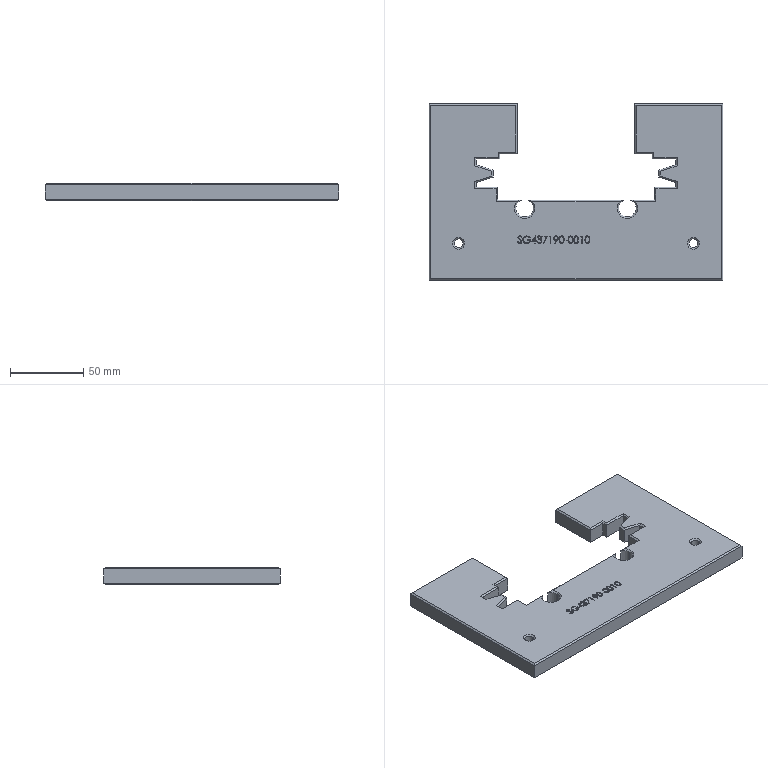Part | STEP file | Rotor mis-part check fixture-go gauge 1 | 1 solid | 285 faces | box 200 x 120 x 12 mm | volume 206238 mm3 | plane 158 | spline 83 | cone 26 | cylinder 18 | commonest cylinder face diameters 1.6 x8 12 x6 6 x4